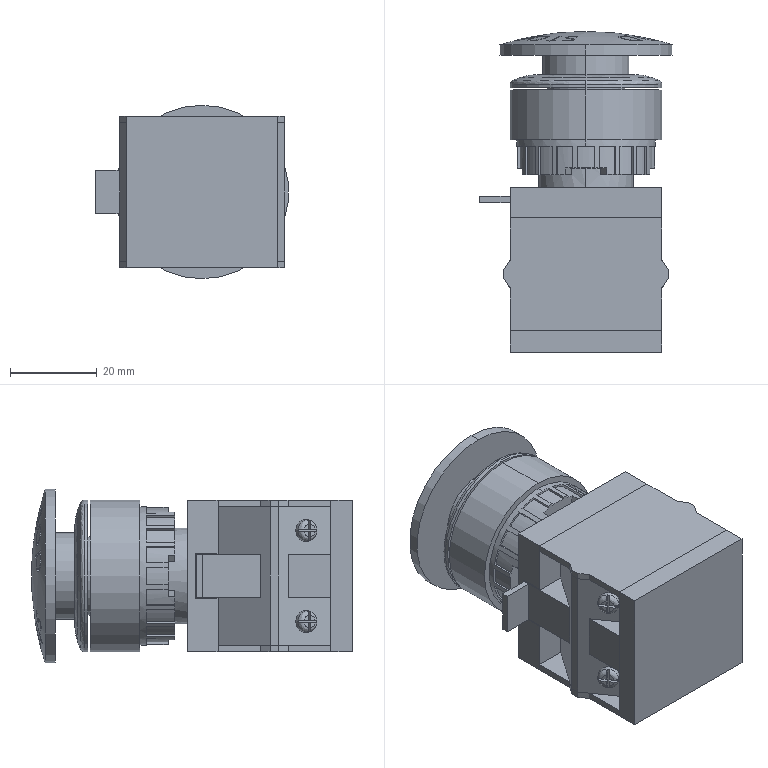Part | SolidWorks | features BaseBody 5 | 5 solids | 484 faces | box 44.5 x 74 x 40 mm | volume 70679 mm3 | plane 316 | spline 121 | cylinder 45 | cone 2 | commonest cylinder face diameters 31 x21 5 x8 35 x4 18 x2 20 x2 20.5 x2